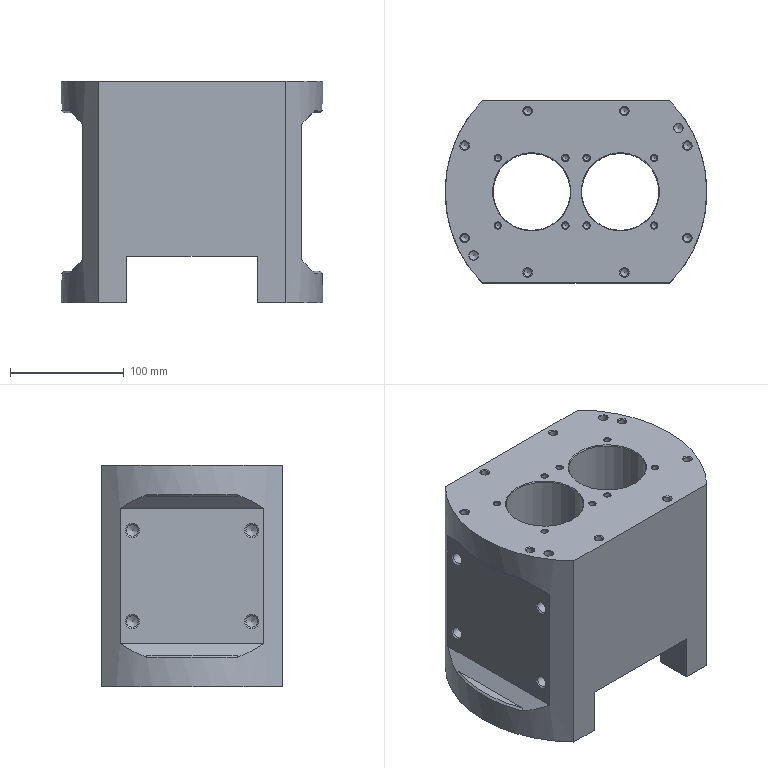NC program | NX | posted with a generic post | part box 230 x 160 x 195 mm
Lines 133 to 1425 of 1674, first 1007 of 1289 lines:
(HOLE_MILLING , TOOL : D35R.5)
N228 T09 M6
N230 G54
N232 G17 G0 G90 X-39. Y0. B0. C0. S1500 M3
N234 G43 Z30. H9
N236 Z1.
N238 G94 G3 X-30.825 Y-8.175 R8.175 F1200.
N240 X-22.65 Y0. R8.175
N242 X-22.65 Y0. Z0.75 I-16.35 J0.
N244 X-22.65 Y0. Z0.5 I-16.35 J0.
N246 X-22.65 Y0. Z0.25 I-16.35 J0.
N248 X-22.65 Y0. Z0. I-16.35 J0.
N250 X-22.65 Y0. Z-0.25 I-16.35 J0.
N252 X-22.65 Y0. Z-0.5 I-16.35 J0.
N254 X-22.65 Y0. Z-0.75 I-16.35 J0.
N256 X-22.65 Y0. Z-1. I-16.35 J0.
N258 X-22.65 Y0. Z-1.25 I-16.35 J0.
N260 X-22.65 Y0. Z-1.5 I-16.35 J0.
N262 X-22.65 Y0. Z-1.75 I-16.35 J0.
N264 X-22.65 Y0. Z-2. I-16.35 J0.
N266 X-22.65 Y0. Z-2.25 I-16.35 J0.
N268 X-22.65 Y0. Z-2.5 I-16.35 J0.
N270 X-22.65 Y0. Z-2.75 I-16.35 J0.
N272 X-22.65 Y0. Z-3. I-16.35 J0.
N274 X-22.65 Y0. Z-3.25 I-16.35 J0.
N276 X-22.65 Y0. Z-3.5 I-16.35 J0.
N278 X-22.65 Y0. Z-3.75 I-16.35 J0.
N280 X-22.65 Y0. Z-4. I-16.35 J0.
N282 X-22.65 Y0. Z-4.25 I-16.35 J0.
N284 X-22.65 Y0. Z-4.5 I-16.35 J0.
N286 X-22.65 Y0. Z-4.75 I-16.35 J0.
N288 X-22.65 Y0. Z-5. I-16.35 J0.
N290 X-22.65 Y0. Z-5.25 I-16.35 J0.
N292 X-22.65 Y0. Z-5.5 I-16.35 J0.
N294 X-22.65 Y0. Z-5.75 I-16.35 J0.
N296 X-22.65 Y0. Z-6. I-16.35 J0.
N298 X-22.65 Y0. Z-6.25 I-16.35 J0.
N300 X-22.65 Y0. Z-6.5 I-16.35 J0.
N302 X-22.65 Y0. Z-6.75 I-16.35 J0.
N304 X-22.65 Y0. Z-7. I-16.35 J0.
N306 X-22.65 Y0. Z-7.25 I-16.35 J0.
N308 X-22.65 Y0. Z-7.5 I-16.35 J0.
N310 X-22.65 Y0. Z-7.75 I-16.35 J0.
N312 X-22.65 Y0. Z-8. I-16.35 J0.
N314 X-22.65 Y0. Z-8.25 I-16.35 J0.
N316 X-22.65 Y0. Z-8.5 I-16.35 J0.
N318 X-22.65 Y0. Z-8.75 I-16.35 J0.
N320 X-22.65 Y0. Z-9. I-16.35 J0.
N322 X-22.65 Y0. Z-9.25 I-16.35 J0.
N324 X-22.65 Y0. Z-9.5 I-16.35 J0.
N326 X-22.65 Y0. Z-9.75 I-16.35 J0.
N328 X-22.65 Y0. Z-10. I-16.35 J0.
N330 X-22.65 Y0. Z-10.25 I-16.35 J0.
N332 X-22.65 Y0. Z-10.5 I-16.35 J0.
N334 X-22.65 Y0. Z-10.75 I-16.35 J0.
N336 X-22.65 Y0. Z-11. I-16.35 J0.
N338 X-22.65 Y0. Z-11.25 I-16.35 J0.
N340 X-22.65 Y0. Z-11.5 I-16.35 J0.
N342 X-22.65 Y0. Z-11.75 I-16.35 J0.
N344 X-22.65 Y0. Z-12. I-16.35 J0.
N346 X-22.65 Y0. Z-12.25 I-16.35 J0.
N348 X-22.65 Y0. Z-12.5 I-16.35 J0.
N350 X-22.65 Y0. Z-12.75 I-16.35 J0.
N352 X-22.65 Y0. Z-13. I-16.35 J0.
N354 X-22.65 Y0. Z-13.25 I-16.35 J0.
N356 X-22.65 Y0. Z-13.5 I-16.35 J0.
N358 X-22.65 Y0. Z-13.75 I-16.35 J0.
N360 X-22.65 Y0. Z-14. I-16.35 J0.
N362 X-22.65 Y0. Z-14.25 I-16.35 J0.
N364 X-22.65 Y0. Z-14.5 I-16.35 J0.
N366 X-22.65 Y0. Z-14.75 I-16.35 J0.
N368 X-22.65 Y0. Z-15. I-16.35 J0.
N370 X-22.65 Y0. Z-15.25 I-16.35 J0.
N372 X-22.65 Y0. Z-15.5 I-16.35 J0.
N374 X-22.65 Y0. Z-15.75 I-16.35 J0.
N376 X-22.65 Y0. Z-16. I-16.35 J0.
N378 X-22.65 Y0. Z-16.25 I-16.35 J0.
N380 X-22.65 Y0. Z-16.5 I-16.35 J0.
N382 X-22.65 Y0. Z-16.75 I-16.35 J0.
N384 X-22.65 Y0. Z-17. I-16.35 J0.
N386 X-22.65 Y0. Z-17.25 I-16.35 J0.
N388 X-22.65 Y0. Z-17.5 I-16.35 J0.
N390 X-22.65 Y0. Z-17.75 I-16.35 J0.
N392 X-22.65 Y0. Z-18. I-16.35 J0.
N394 X-22.65 Y0. Z-18.25 I-16.35 J0.
N396 X-22.65 Y0. Z-18.5 I-16.35 J0.
N398 X-22.65 Y0. Z-18.75 I-16.35 J0.
N400 X-22.65 Y0. Z-19. I-16.35 J0.
N402 X-22.65 Y0. Z-19.25 I-16.35 J0.
N404 X-22.65 Y0. Z-19.5 I-16.35 J0.
N406 X-22.65 Y0. Z-19.75 I-16.35 J0.
N408 X-22.65 Y0. Z-20. I-16.35 J0.
N410 X-22.65 Y0. Z-20.25 I-16.35 J0.
N412 X-22.65 Y0. Z-20.5 I-16.35 J0.
N414 X-22.65 Y0. Z-20.75 I-16.35 J0.
N416 X-22.65 Y0. Z-21. I-16.35 J0.
N418 X-22.65 Y0. Z-21.25 I-16.35 J0.
N420 X-22.65 Y0. Z-21.5 I-16.35 J0.
N422 X-22.65 Y0. Z-21.75 I-16.35 J0.
N424 X-22.65 Y0. Z-22. I-16.35 J0.
N426 X-22.65 Y0. Z-22.25 I-16.35 J0.
N428 X-22.65 Y0. Z-22.5 I-16.35 J0.
N430 X-22.65 Y0. Z-22.75 I-16.35 J0.
N432 X-22.65 Y0. Z-23. I-16.35 J0.
N434 X-22.65 Y0. Z-23.25 I-16.35 J0.
N436 X-22.65 Y0. Z-23.5 I-16.35 J0.
N438 X-22.65 Y0. Z-23.75 I-16.35 J0.
N440 X-22.65 Y0. Z-24. I-16.35 J0.
N442 X-22.65 Y0. Z-24.25 I-16.35 J0.
N444 X-22.65 Y0. Z-24.5 I-16.35 J0.
N446 X-22.65 Y0. Z-24.75 I-16.35 J0.
N448 X-22.65 Y0. Z-25. I-16.35 J0.
N450 X-22.65 Y0. Z-25.25 I-16.35 J0.
N452 X-22.65 Y0. Z-25.5 I-16.35 J0.
N454 X-22.65 Y0. Z-25.75 I-16.35 J0.
N456 X-22.65 Y0. Z-26. I-16.35 J0.
N458 X-22.65 Y0. Z-26.25 I-16.35 J0.
N460 X-22.65 Y0. Z-26.5 I-16.35 J0.
N462 X-22.65 Y0. Z-26.75 I-16.35 J0.
N464 X-22.65 Y0. Z-27. I-16.35 J0.
N466 X-22.65 Y0. Z-27.25 I-16.35 J0.
N468 X-22.65 Y0. Z-27.5 I-16.35 J0.
N470 X-22.65 Y0. Z-27.75 I-16.35 J0.
N472 X-22.65 Y0. Z-28. I-16.35 J0.
N474 X-22.65 Y0. Z-28.25 I-16.35 J0.
N476 X-22.65 Y0. Z-28.5 I-16.35 J0.
N478 X-22.65 Y0. Z-28.75 I-16.35 J0.
N480 X-22.65 Y0. Z-29. I-16.35 J0.
N482 X-22.65 Y0. Z-29.25 I-16.35 J0.
N484 X-22.65 Y0. Z-29.5 I-16.35 J0.
N486 X-22.65 Y0. Z-29.75 I-16.35 J0.
N488 X-22.65 Y0. Z-30. I-16.35 J0.
N490 X-22.65 Y0. Z-30.25 I-16.35 J0.
N492 X-22.65 Y0. Z-30.5 I-16.35 J0.
N494 X-22.65 Y0. Z-30.75 I-16.35 J0.
N496 X-22.65 Y0. Z-31. I-16.35 J0.
N498 X-22.65 Y0. Z-31.25 I-16.35 J0.
N500 X-22.65 Y0. Z-31.5 I-16.35 J0.
N502 X-22.65 Y0. Z-31.75 I-16.35 J0.
N504 X-22.65 Y0. Z-32. I-16.35 J0.
N506 X-22.65 Y0. Z-32.25 I-16.35 J0.
N508 X-22.65 Y0. Z-32.5 I-16.35 J0.
N510 X-22.65 Y0. Z-32.75 I-16.35 J0.
N512 X-22.65 Y0. Z-33. I-16.35 J0.
N514 X-22.65 Y0. Z-33.25 I-16.35 J0.
N516 X-22.65 Y0. Z-33.5 I-16.35 J0.
N518 X-22.65 Y0. Z-33.75 I-16.35 J0.
N520 X-22.65 Y0. Z-34. I-16.35 J0.
N522 X-22.65 Y0. Z-34.25 I-16.35 J0.
N524 X-22.65 Y0. Z-34.5 I-16.35 J0.
N526 X-22.65 Y0. Z-34.75 I-16.35 J0.
N528 X-22.65 Y0. Z-35. I-16.35 J0.
N530 X-22.65 Y0. Z-35.25 I-16.35 J0.
N532 X-22.65 Y0. Z-35.5 I-16.35 J0.
N534 X-22.65 Y0. Z-35.75 I-16.35 J0.
N536 X-22.65 Y0. Z-36. I-16.35 J0.
N538 X-22.65 Y0. Z-36.25 I-16.35 J0.
N540 X-22.65 Y0. Z-36.5 I-16.35 J0.
N542 X-22.65 Y0. Z-36.75 I-16.35 J0.
N544 X-22.65 Y0. Z-37. I-16.35 J0.
N546 X-22.65 Y0. Z-37.25 I-16.35 J0.
N548 X-22.65 Y0. Z-37.5 I-16.35 J0.
N550 X-22.65 Y0. Z-37.75 I-16.35 J0.
N552 X-22.65 Y0. Z-38. I-16.35 J0.
N554 X-22.65 Y0. Z-38.25 I-16.35 J0.
N556 X-22.65 Y0. Z-38.5 I-16.35 J0.
N558 X-22.65 Y0. Z-38.75 I-16.35 J0.
N560 X-22.65 Y0. Z-39. I-16.35 J0.
N562 X-22.65 Y0. Z-39.25 I-16.35 J0.
N564 X-22.65 Y0. Z-39.5 I-16.35 J0.
N566 X-22.65 Y0. Z-39.75 I-16.35 J0.
N568 X-22.65 Y0. Z-40. I-16.35 J0.
N570 X-22.65 Y0. Z-40.25 I-16.35 J0.
N572 X-22.65 Y0. Z-40.5 I-16.35 J0.
N574 X-22.65 Y0. Z-40.75 I-16.35 J0.
N576 X-22.65 Y0. Z-41. I-16.35 J0.
N578 X-22.65 Y0. Z-41.25 I-16.35 J0.
N580 X-22.65 Y0. Z-41.5 I-16.35 J0.
N582 X-22.65 Y0. Z-41.75 I-16.35 J0.
N584 X-22.65 Y0. Z-42. I-16.35 J0.
N586 X-22.65 Y0. Z-42.25 I-16.35 J0.
N588 X-22.65 Y0. Z-42.5 I-16.35 J0.
N590 X-22.65 Y0. Z-42.75 I-16.35 J0.
N592 X-22.65 Y0. Z-43. I-16.35 J0.
N594 X-22.65 Y0. Z-43.25 I-16.35 J0.
N596 X-22.65 Y0. Z-43.5 I-16.35 J0.
N598 X-22.65 Y0. Z-43.75 I-16.35 J0.
N600 X-22.65 Y0. Z-44. I-16.35 J0.
N602 X-22.65 Y0. Z-44.25 I-16.35 J0.
N604 X-22.65 Y0. Z-44.5 I-16.35 J0.
N606 X-22.65 Y0. Z-44.75 I-16.35 J0.
N608 X-22.65 Y0. Z-45. I-16.35 J0.
N610 X-22.65 Y0. Z-45.25 I-16.35 J0.
N612 X-22.65 Y0. Z-45.5 I-16.35 J0.
N614 X-22.65 Y0. Z-45.75 I-16.35 J0.
N616 X-22.65 Y0. Z-46. I-16.35 J0.
N618 X-22.65 Y0. Z-46.25 I-16.35 J0.
N620 X-22.65 Y0. Z-46.5 I-16.35 J0.
N622 X-22.65 Y0. Z-46.75 I-16.35 J0.
N624 X-22.65 Y0. Z-47. I-16.35 J0.
N626 X-22.65 Y0. Z-47.25 I-16.35 J0.
N628 X-22.65 Y0. Z-47.5 I-16.35 J0.
N630 X-22.65 Y0. Z-47.75 I-16.35 J0.
N632 X-22.65 Y0. Z-48. I-16.35 J0.
N634 X-22.65 Y0. Z-48.25 I-16.35 J0.
N636 X-22.65 Y0. Z-48.5 I-16.35 J0.
N638 X-22.65 Y0. Z-48.75 I-16.35 J0.
N640 X-22.65 Y0. Z-49. I-16.35 J0.
N642 X-22.65 Y0. Z-49.25 I-16.35 J0.
N644 X-22.65 Y0. Z-49.5 I-16.35 J0.
N646 X-22.65 Y0. Z-49.75 I-16.35 J0.
N648 X-22.65 Y0. Z-50. I-16.35 J0.
N650 X-22.65 Y0. Z-50.25 I-16.35 J0.
N652 X-22.65 Y0. Z-50.5 I-16.35 J0.
N654 X-22.65 Y0. Z-50.75 I-16.35 J0.
N656 X-22.65 Y0. Z-51. I-16.35 J0.
N658 X-22.65 Y0. Z-51.25 I-16.35 J0.
N660 X-22.65 Y0. Z-51.5 I-16.35 J0.
N662 X-22.65 Y0. Z-51.75 I-16.35 J0.
N664 X-22.65 Y0. Z-52. I-16.35 J0.
N666 X-22.65 Y0. Z-52.25 I-16.35 J0.
N668 X-22.65 Y0. Z-52.5 I-16.35 J0.
N670 X-22.65 Y0. Z-52.75 I-16.35 J0.
N672 X-22.65 Y0. Z-53. I-16.35 J0.
N674 X-22.65 Y0. Z-53.25 I-16.35 J0.
N676 X-22.65 Y0. Z-53.5 I-16.35 J0.
N678 X-22.65 Y0. Z-53.75 I-16.35 J0.
N680 X-22.65 Y0. Z-54. I-16.35 J0.
N682 X-22.65 Y0. Z-54.25 I-16.35 J0.
N684 X-22.65 Y0. Z-54.5 I-16.35 J0.
N686 X-22.65 Y0. Z-54.75 I-16.35 J0.
N688 X-22.65 Y0. Z-55. I-16.35 J0.
N690 X-22.65 Y0. Z-55.25 I-16.35 J0.
N692 X-22.65 Y0. Z-55.5 I-16.35 J0.
N694 X-22.65 Y0. Z-55.75 I-16.35 J0.
N696 X-22.65 Y0. Z-56. I-16.35 J0.
N698 X-22.65 Y0. Z-56.25 I-16.35 J0.
N700 X-22.65 Y0. Z-56.5 I-16.35 J0.
N702 X-22.65 Y0. Z-56.75 I-16.35 J0.
N704 X-22.65 Y0. Z-57. I-16.35 J0.
N706 X-22.65 Y0. Z-57.25 I-16.35 J0.
N708 X-22.65 Y0. Z-57.5 I-16.35 J0.
N710 X-22.65 Y0. Z-57.75 I-16.35 J0.
N712 X-22.65 Y0. Z-58. I-16.35 J0.
N714 X-22.65 Y0. Z-58.25 I-16.35 J0.
N716 X-22.65 Y0. Z-58.5 I-16.35 J0.
N718 X-22.65 Y0. Z-58.75 I-16.35 J0.
N720 X-22.65 Y0. Z-59. I-16.35 J0.
N722 X-22.65 Y0. Z-59.25 I-16.35 J0.
N724 X-22.65 Y0. Z-59.5 I-16.35 J0.
N726 X-22.65 Y0. Z-59.75 I-16.35 J0.
N728 X-22.65 Y0. Z-60. I-16.35 J0.
N730 X-22.65 Y0. Z-60.25 I-16.35 J0.
N732 X-22.65 Y0. Z-60.5 I-16.35 J0.
N734 X-22.65 Y0. Z-60.75 I-16.35 J0.
N736 X-22.65 Y0. Z-61. I-16.35 J0.
N738 X-22.65 Y0. Z-61.25 I-16.35 J0.
N740 X-22.65 Y0. Z-61.5 I-16.35 J0.
N742 X-22.65 Y0. Z-61.75 I-16.35 J0.
N744 X-22.65 Y0. Z-62. I-16.35 J0.
N746 X-22.65 Y0. Z-62.25 I-16.35 J0.
N748 X-22.65 Y0. Z-62.5 I-16.35 J0.
N750 X-22.65 Y0. Z-62.75 I-16.35 J0.
N752 X-22.65 Y0. Z-63. I-16.35 J0.
N754 X-22.65 Y0. Z-63.25 I-16.35 J0.
N756 X-22.65 Y0. Z-63.5 I-16.35 J0.
N758 X-22.65 Y0. Z-63.75 I-16.35 J0.
N760 X-22.65 Y0. Z-64. I-16.35 J0.
N762 X-22.65 Y0. Z-64.25 I-16.35 J0.
N764 X-22.65 Y0. Z-64.5 I-16.35 J0.
N766 X-22.65 Y0. Z-64.75 I-16.35 J0.
N768 X-22.65 Y0. Z-65. I-16.35 J0.
N770 X-22.65 Y0. Z-65.25 I-16.35 J0.
N772 X-22.65 Y0. Z-65.5 I-16.35 J0.
N774 X-22.65 Y0. Z-65.75 I-16.35 J0.
N776 X-22.65 Y0. Z-66. I-16.35 J0.
N778 X-22.65 Y0. Z-66.25 I-16.35 J0.
N780 X-22.65 Y0. Z-66.5 I-16.35 J0.
N782 X-22.65 Y0. Z-66.75 I-16.35 J0.
N784 X-22.65 Y0. Z-67. I-16.35 J0.
N786 X-22.65 Y0. Z-67.25 I-16.35 J0.
N788 X-22.65 Y0. Z-67.5 I-16.35 J0.
N790 X-22.65 Y0. Z-67.75 I-16.35 J0.
N792 X-22.65 Y0. Z-68. I-16.35 J0.
N794 X-22.65 Y0. Z-68.25 I-16.35 J0.
N796 X-22.65 Y0. Z-68.5 I-16.35 J0.
N798 X-22.65 Y0. Z-68.75 I-16.35 J0.
N800 X-22.65 Y0. Z-69. I-16.35 J0.
N802 X-22.65 Y0. Z-69.25 I-16.35 J0.
N804 X-22.65 Y0. Z-69.5 I-16.35 J0.
N806 X-22.65 Y0. Z-69.75 I-16.35 J0.
N808 X-22.65 Y0. Z-70. I-16.35 J0.
N810 X-22.65 Y0. Z-70.25 I-16.35 J0.
N812 X-22.65 Y0. Z-70.5 I-16.35 J0.
N814 X-22.65 Y0. Z-70.75 I-16.35 J0.
N816 X-22.65 Y0. Z-71. I-16.35 J0.
N818 X-22.65 Y0. Z-71.25 I-16.35 J0.
N820 X-22.65 Y0. Z-71.5 I-16.35 J0.
N822 X-22.65 Y0. Z-71.75 I-16.35 J0.
N824 X-22.65 Y0. Z-72. I-16.35 J0.
N826 X-22.65 Y0. Z-72.25 I-16.35 J0.
N828 X-22.65 Y0. Z-72.5 I-16.35 J0.
N830 X-22.65 Y0. Z-72.75 I-16.35 J0.
N832 X-22.65 Y0. Z-73. I-16.35 J0.
N834 X-22.65 Y0. Z-73.25 I-16.35 J0.
N836 X-22.65 Y0. Z-73.5 I-16.35 J0.
N838 X-22.65 Y0. Z-73.75 I-16.35 J0.
N840 X-22.65 Y0. Z-74. I-16.35 J0.
N842 X-22.65 Y0. Z-74.25 I-16.35 J0.
N844 X-22.65 Y0. Z-74.5 I-16.35 J0.
N846 X-22.65 Y0. Z-74.75 I-16.35 J0.
N848 X-22.65 Y0. Z-75. I-16.35 J0.
N850 X-22.65 Y0. Z-75.25 I-16.35 J0.
N852 X-22.65 Y0. Z-75.5 I-16.35 J0.
N854 X-22.65 Y0. Z-75.75 I-16.35 J0.
N856 X-22.65 Y0. Z-76. I-16.35 J0.
N858 X-22.65 Y0. Z-76.25 I-16.35 J0.
N860 X-22.65 Y0. Z-76.5 I-16.35 J0.
N862 X-22.65 Y0. Z-76.75 I-16.35 J0.
N864 X-22.65 Y0. Z-77. I-16.35 J0.
N866 X-22.65 Y0. Z-77.25 I-16.35 J0.
N868 X-22.65 Y0. Z-77.5 I-16.35 J0.
N870 X-22.65 Y0. Z-77.75 I-16.35 J0.
N872 X-22.65 Y0. Z-78. I-16.35 J0.
N874 X-22.65 Y0. Z-78.25 I-16.35 J0.
N876 X-22.65 Y0. Z-78.5 I-16.35 J0.
N878 X-22.65 Y0. Z-78.75 I-16.35 J0.
N880 X-22.65 Y0. Z-79. I-16.35 J0.
N882 X-22.65 Y0. Z-79.25 I-16.35 J0.
N884 X-22.65 Y0. Z-79.5 I-16.35 J0.
N886 X-22.65 Y0. Z-79.75 I-16.35 J0.
N888 X-22.65 Y0. Z-80. I-16.35 J0.
N890 X-22.65 Y0. Z-80.25 I-16.35 J0.
N892 X-22.65 Y0. Z-80.5 I-16.35 J0.
N894 X-22.65 Y0. Z-80.75 I-16.35 J0.
N896 X-22.65 Y0. Z-81. I-16.35 J0.
N898 X-22.65 Y0. Z-81.25 I-16.35 J0.
N900 X-22.65 Y0. Z-81.5 I-16.35 J0.
N902 X-22.65 Y0. Z-81.75 I-16.35 J0.
N904 X-22.65 Y0. Z-82. I-16.35 J0.
N906 X-22.65 Y0. Z-82.25 I-16.35 J0.
N908 X-22.65 Y0. Z-82.5 I-16.35 J0.
N910 X-22.65 Y0. Z-82.75 I-16.35 J0.
N912 X-22.65 Y0. Z-83. I-16.35 J0.
N914 X-22.65 Y0. Z-83.25 I-16.35 J0.
N916 X-22.65 Y0. Z-83.5 I-16.35 J0.
N918 X-22.65 Y0. Z-83.75 I-16.35 J0.
N920 X-22.65 Y0. Z-84. I-16.35 J0.
N922 X-22.65 Y0. Z-84.25 I-16.35 J0.
N924 X-22.65 Y0. Z-84.5 I-16.35 J0.
N926 X-22.65 Y0. Z-84.75 I-16.35 J0.
N928 X-22.65 Y0. Z-85. I-16.35 J0.
N930 X-22.65 Y0. Z-85.25 I-16.35 J0.
N932 X-22.65 Y0. Z-85.5 I-16.35 J0.
N934 X-22.65 Y0. Z-85.75 I-16.35 J0.
N936 X-22.65 Y0. Z-86. I-16.35 J0.
N938 X-22.65 Y0. Z-86.25 I-16.35 J0.
N940 X-22.65 Y0. Z-86.5 I-16.35 J0.
N942 X-22.65 Y0. Z-86.75 I-16.35 J0.
N944 X-22.65 Y0. Z-87. I-16.35 J0.
N946 X-22.65 Y0. Z-87.25 I-16.35 J0.
N948 X-22.65 Y0. Z-87.5 I-16.35 J0.
N950 X-22.65 Y0. Z-87.75 I-16.35 J0.
N952 X-22.65 Y0. Z-88. I-16.35 J0.
N954 X-22.65 Y0. Z-88.25 I-16.35 J0.
N956 X-22.65 Y0. Z-88.5 I-16.35 J0.
N958 X-22.65 Y0. Z-88.75 I-16.35 J0.
N960 X-22.65 Y0. Z-89. I-16.35 J0.
N962 X-22.65 Y0. Z-89.25 I-16.35 J0.
N964 X-22.65 Y0. Z-89.5 I-16.35 J0.
N966 X-22.65 Y0. Z-89.75 I-16.35 J0.
N968 X-22.65 Y0. Z-90. I-16.35 J0.
N970 X-22.65 Y0. Z-90.25 I-16.35 J0.
N972 X-22.65 Y0. Z-90.5 I-16.35 J0.
N974 X-22.65 Y0. Z-90.75 I-16.35 J0.
N976 X-22.65 Y0. Z-91. I-16.35 J0.
N978 X-22.65 Y0. Z-91.25 I-16.35 J0.
N980 X-22.65 Y0. Z-91.5 I-16.35 J0.
N982 X-22.65 Y0. Z-91.75 I-16.35 J0.
N984 X-22.65 Y0. Z-92. I-16.35 J0.
N986 X-22.65 Y0. Z-92.25 I-16.35 J0.
N988 X-22.65 Y0. Z-92.5 I-16.35 J0.
N990 X-22.65 Y0. Z-92.75 I-16.35 J0.
N992 X-22.65 Y0. Z-93. I-16.35 J0.
N994 X-22.65 Y0. Z-93.25 I-16.35 J0.
N996 X-22.65 Y0. Z-93.5 I-16.35 J0.
N998 X-22.65 Y0. Z-93.75 I-16.35 J0.
N1000 X-22.65 Y0. Z-94. I-16.35 J0.
N1002 X-22.65 Y0. Z-94.25 I-16.35 J0.
N1004 X-22.65 Y0. Z-94.5 I-16.35 J0.
N1006 X-22.65 Y0. Z-94.75 I-16.35 J0.
N1008 X-22.65 Y0. Z-95. I-16.35 J0.
N1010 X-22.65 Y0. Z-95.25 I-16.35 J0.
N1012 X-22.65 Y0. Z-95.5 I-16.35 J0.
N1014 X-22.65 Y0. Z-95.75 I-16.35 J0.
N1016 X-22.65 Y0. Z-96. I-16.35 J0.
N1018 X-22.65 Y0. Z-96.25 I-16.35 J0.
N1020 X-22.65 Y0. Z-96.5 I-16.35 J0.
N1022 X-22.65 Y0. Z-96.75 I-16.35 J0.
N1024 X-22.65 Y0. Z-97. I-16.35 J0.
N1026 X-22.65 Y0. Z-97.25 I-16.35 J0.
N1028 X-22.65 Y0. Z-97.5 I-16.35 J0.
N1030 X-22.65 Y0. Z-97.75 I-16.35 J0.
N1032 X-22.65 Y0. Z-98. I-16.35 J0.
N1034 X-22.65 Y0. Z-98.25 I-16.35 J0.
N1036 X-22.65 Y0. Z-98.5 I-16.35 J0.
N1038 X-22.65 Y0. Z-98.75 I-16.35 J0.
N1040 X-22.65 Y0. Z-99. I-16.35 J0.
N1042 X-22.65 Y0. Z-99.25 I-16.35 J0.
N1044 X-22.65 Y0. Z-99.5 I-16.35 J0.
N1046 X-22.65 Y0. Z-99.75 I-16.35 J0.
N1048 X-22.65 Y0. Z-100. I-16.35 J0.
N1050 X-22.65 Y0. Z-100.25 I-16.35 J0.
N1052 X-22.65 Y0. Z-100.5 I-16.35 J0.
N1054 X-22.65 Y0. Z-100.75 I-16.35 J0.
N1056 X-22.65 Y0. Z-101. I-16.35 J0.
N1058 X-22.65 Y0. Z-101.25 I-16.35 J0.
N1060 X-22.65 Y0. Z-101.5 I-16.35 J0.
N1062 X-22.65 Y0. Z-101.75 I-16.35 J0.
N1064 X-22.65 Y0. Z-102. I-16.35 J0.
N1066 X-22.65 Y0. Z-102.25 I-16.35 J0.
N1068 X-22.65 Y0. Z-102.5 I-16.35 J0.
N1070 X-22.65 Y0. Z-102.75 I-16.35 J0.
N1072 X-22.65 Y0. Z-103. I-16.35 J0.
N1074 X-22.65 Y0. Z-103.25 I-16.35 J0.
N1076 X-22.65 Y0. Z-103.5 I-16.35 J0.
N1078 X-22.65 Y0. Z-103.75 I-16.35 J0.
N1080 X-22.65 Y0. Z-104. I-16.35 J0.
N1082 X-22.65 Y0. Z-104.25 I-16.35 J0.
N1084 X-22.65 Y0. Z-104.5 I-16.35 J0.
N1086 X-22.65 Y0. Z-104.75 I-16.35 J0.
N1088 X-22.65 Y0. Z-105. I-16.35 J0.
N1090 X-22.65 Y0. Z-105.25 I-16.35 J0.
N1092 X-22.65 Y0. Z-105.5 I-16.35 J0.
N1094 X-22.65 Y0. Z-105.75 I-16.35 J0.
N1096 X-22.65 Y0. Z-106. I-16.35 J0.
N1098 X-22.65 Y0. Z-106.25 I-16.35 J0.
N1100 X-22.65 Y0. Z-106.5 I-16.35 J0.
N1102 X-22.65 Y0. Z-106.75 I-16.35 J0.
N1104 X-22.65 Y0. Z-107. I-16.35 J0.
N1106 X-22.65 Y0. Z-107.25 I-16.35 J0.
N1108 X-22.65 Y0. Z-107.5 I-16.35 J0.
N1110 X-22.65 Y0. Z-107.75 I-16.35 J0.
N1112 X-22.65 Y0. Z-108. I-16.35 J0.
N1114 X-22.65 Y0. Z-108.25 I-16.35 J0.
N1116 X-22.65 Y0. Z-108.5 I-16.35 J0.
N1118 X-22.65 Y0. Z-108.75 I-16.35 J0.
N1120 X-22.65 Y0. Z-109. I-16.35 J0.
N1122 X-22.65 Y0. Z-109.25 I-16.35 J0.
N1124 X-22.65 Y0. Z-109.5 I-16.35 J0.
N1126 X-22.65 Y0. Z-109.75 I-16.35 J0.
N1128 X-22.65 Y0. Z-110. I-16.35 J0.
N1130 X-22.65 Y0. Z-110.25 I-16.35 J0.
N1132 X-22.65 Y0. Z-110.5 I-16.35 J0.
N1134 X-22.65 Y0. Z-110.75 I-16.35 J0.
N1136 X-22.65 Y0. Z-111. I-16.35 J0.
N1138 X-22.65 Y0. Z-111.25 I-16.35 J0.
N1140 X-22.65 Y0. Z-111.5 I-16.35 J0.
N1142 X-22.65 Y0. Z-111.75 I-16.35 J0.
N1144 X-22.65 Y0. Z-112. I-16.35 J0.
N1146 X-22.65 Y0. Z-112.25 I-16.35 J0.
N1148 X-22.65 Y0. Z-112.5 I-16.35 J0.
N1150 X-22.65 Y0. Z-112.75 I-16.35 J0.
N1152 X-22.65 Y0. Z-113. I-16.35 J0.
N1154 X-22.65 Y0. Z-113.25 I-16.35 J0.
N1156 X-22.65 Y0. Z-113.5 I-16.35 J0.
N1158 X-22.65 Y0. Z-113.75 I-16.35 J0.
N1160 X-22.65 Y0. Z-114. I-16.35 J0.
N1162 X-22.65 Y0. Z-114.25 I-16.35 J0.
N1164 X-22.65 Y0. Z-114.5 I-16.35 J0.
N1166 X-22.65 Y0. Z-114.75 I-16.35 J0.
N1168 X-22.65 Y0. Z-115. I-16.35 J0.
N1170 X-22.65 Y0. Z-115.25 I-16.35 J0.
N1172 X-22.65 Y0. Z-115.5 I-16.35 J0.
N1174 X-22.65 Y0. Z-115.75 I-16.35 J0.
N1176 X-22.65 Y0. Z-116. I-16.35 J0.
N1178 X-22.65 Y0. Z-116.25 I-16.35 J0.
N1180 X-22.65 Y0. Z-116.5 I-16.35 J0.
N1182 X-22.65 Y0. Z-116.75 I-16.35 J0.
N1184 X-22.65 Y0. Z-117. I-16.35 J0.
N1186 X-22.65 Y0. Z-117.25 I-16.35 J0.
N1188 X-22.65 Y0. Z-117.5 I-16.35 J0.
N1190 X-22.65 Y0. Z-117.75 I-16.35 J0.
N1192 X-22.65 Y0. Z-118. I-16.35 J0.
N1194 X-22.65 Y0. Z-118.25 I-16.35 J0.
N1196 X-22.65 Y0. Z-118.5 I-16.35 J0.
N1198 X-22.65 Y0. Z-118.75 I-16.35 J0.
N1200 X-22.65 Y0. Z-119. I-16.35 J0.
N1202 X-22.65 Y0. Z-119.25 I-16.35 J0.
N1204 X-22.65 Y0. Z-119.5 I-16.35 J0.
N1206 X-22.65 Y0. Z-119.75 I-16.35 J0.
N1208 X-22.65 Y0. Z-120. I-16.35 J0.
N1210 X-22.65 Y0. Z-120.25 I-16.35 J0.
N1212 X-22.65 Y0. Z-120.5 I-16.35 J0.
N1214 X-22.65 Y0. Z-120.75 I-16.35 J0.
N1216 X-22.65 Y0. Z-121. I-16.35 J0.
N1218 X-22.65 Y0. Z-121.25 I-16.35 J0.
N1220 X-22.65 Y0. Z-121.5 I-16.35 J0.
N1222 X-22.65 Y0. Z-121.75 I-16.35 J0.
N1224 X-22.65 Y0. Z-122. I-16.35 J0.
N1226 X-22.65 Y0. Z-122.25 I-16.35 J0.
N1228 X-22.65 Y0. Z-122.5 I-16.35 J0.
N1230 X-22.65 Y0. Z-122.75 I-16.35 J0.
N1232 X-22.65 Y0. Z-123. I-16.35 J0.
N1234 X-22.65 Y0. Z-123.25 I-16.35 J0.
N1236 X-22.65 Y0. Z-123.5 I-16.35 J0.
N1238 X-22.65 Y0. Z-123.75 I-16.35 J0.
N1240 X-22.65 Y0. Z-124. I-16.35 J0.
N1242 X-22.65 Y0. Z-124.25 I-16.35 J0.
N1244 X-22.65 Y0. Z-124.5 I-16.35 J0.
N1246 X-22.65 Y0. Z-124.75 I-16.35 J0.
N1248 X-22.65 Y0. Z-125. I-16.35 J0.
N1250 X-22.65 Y0. Z-125.25 I-16.35 J0.
N1252 X-22.65 Y0. Z-125.5 I-16.35 J0.
N1254 X-22.65 Y0. Z-125.75 I-16.35 J0.
N1256 X-22.65 Y0. Z-126. I-16.35 J0.
N1258 X-22.65 Y0. Z-126.25 I-16.35 J0.
N1260 X-22.65 Y0. Z-126.5 I-16.35 J0.
N1262 X-22.65 Y0. Z-126.75 I-16.35 J0.
N1264 X-22.65 Y0. Z-127. I-16.35 J0.
N1266 X-22.65 Y0. Z-127.25 I-16.35 J0.
N1268 X-22.65 Y0. Z-127.5 I-16.35 J0.
N1270 X-22.65 Y0. Z-127.75 I-16.35 J0.
N1272 X-22.65 Y0. Z-128. I-16.35 J0.
N1274 X-22.65 Y0. Z-128.25 I-16.35 J0.
N1276 X-22.65 Y0. Z-128.5 I-16.35 J0.
N1278 X-22.65 Y0. Z-128.75 I-16.35 J0.
N1280 X-22.65 Y0. Z-129. I-16.35 J0.
N1282 X-22.65 Y0. Z-129.25 I-16.35 J0.
N1284 X-22.65 Y0. Z-129.5 I-16.35 J0.
N1286 X-22.65 Y0. Z-129.75 I-16.35 J0.
N1288 X-22.65 Y0. Z-130. I-16.35 J0.
N1290 X-22.65 Y0. Z-130.25 I-16.35 J0.
N1292 X-22.65 Y0. Z-130.5 I-16.35 J0.
N1294 X-22.65 Y0. Z-130.75 I-16.35 J0.
N1296 X-22.65 Y0. Z-131. I-16.35 J0.
N1298 X-22.65 Y0. Z-131.25 I-16.35 J0.
N1300 X-22.65 Y0. Z-131.5 I-16.35 J0.
N1302 X-22.65 Y0. Z-131.75 I-16.35 J0.
N1304 X-22.65 Y0. Z-132. I-16.35 J0.
N1306 X-22.65 Y0. Z-132.25 I-16.35 J0.
N1308 X-22.65 Y0. Z-132.5 I-16.35 J0.
N1310 X-22.65 Y0. Z-132.75 I-16.35 J0.
N1312 X-22.65 Y0. Z-133. I-16.35 J0.
N1314 X-22.65 Y0. Z-133.25 I-16.35 J0.
N1316 X-22.65 Y0. Z-133.5 I-16.35 J0.
N1318 X-22.65 Y0. Z-133.75 I-16.35 J0.
N1320 X-22.65 Y0. Z-134. I-16.35 J0.
N1322 X-22.65 Y0. Z-134.25 I-16.35 J0.
N1324 X-22.65 Y0. Z-134.5 I-16.35 J0.
N1326 X-22.65 Y0. Z-134.75 I-16.35 J0.
N1328 X-22.65 Y0. Z-135. I-16.35 J0.
N1330 X-22.65 Y0. Z-135.25 I-16.35 J0.
N1332 X-22.65 Y0. Z-135.5 I-16.35 J0.
N1334 X-22.65 Y0. Z-135.75 I-16.35 J0.
N1336 X-22.65 Y0. Z-136. I-16.35 J0.
N1338 X-22.65 Y0. Z-136.25 I-16.35 J0.
N1340 X-22.65 Y0. Z-136.5 I-16.35 J0.
N1342 X-22.65 Y0. Z-136.75 I-16.35 J0.
N1344 X-22.65 Y0. Z-137. I-16.35 J0.
N1346 X-22.65 Y0. Z-137.25 I-16.35 J0.
N1348 X-22.65 Y0. Z-137.5 I-16.35 J0.
N1350 X-22.65 Y0. Z-137.75 I-16.35 J0.
N1352 X-22.65 Y0. Z-138. I-16.35 J0.
N1354 X-22.65 Y0. Z-138.25 I-16.35 J0.
N1356 X-22.65 Y0. Z-138.5 I-16.35 J0.
N1358 X-22.65 Y0. Z-138.75 I-16.35 J0.
N1360 X-22.65 Y0. Z-139. I-16.35 J0.
N1362 X-22.65 Y0. Z-139.25 I-16.35 J0.
N1364 X-22.65 Y0. Z-139.5 I-16.35 J0.
N1366 X-22.65 Y0. Z-139.75 I-16.35 J0.
N1368 X-22.65 Y0. Z-140. I-16.35 J0.
N1370 X-22.65 Y0. Z-140.25 I-16.35 J0.
N1372 X-22.65 Y0. Z-140.5 I-16.35 J0.
N1374 X-22.65 Y0. Z-140.75 I-16.35 J0.
N1376 X-22.65 Y0. Z-141. I-16.35 J0.
N1378 X-22.65 Y0. Z-141.25 I-16.35 J0.
N1380 X-22.65 Y0. Z-141.5 I-16.35 J0.
N1382 X-22.65 Y0. Z-141.75 I-16.35 J0.
N1384 X-22.65 Y0. Z-142. I-16.35 J0.
N1386 X-22.65 Y0. Z-142.25 I-16.35 J0.
N1388 X-22.65 Y0. Z-142.5 I-16.35 J0.
N1390 X-22.65 Y0. Z-142.75 I-16.35 J0.
N1392 X-22.65 Y0. Z-143. I-16.35 J0.
N1394 X-22.65 Y0. Z-143.25 I-16.35 J0.
N1396 X-22.65 Y0. Z-143.5 I-16.35 J0.
N1398 X-22.65 Y0. Z-143.75 I-16.35 J0.
N1400 X-22.65 Y0. Z-144. I-16.35 J0.
N1402 X-22.65 Y0. Z-144.25 I-16.35 J0.
N1404 X-22.65 Y0. Z-144.5 I-16.35 J0.
N1406 X-22.65 Y0. Z-144.75 I-16.35 J0.
N1408 X-22.65 Y0. Z-145. I-16.35 J0.
N1410 X-22.65 Y0. Z-145.25 I-16.35 J0.
N1412 X-22.65 Y0. Z-145.5 I-16.35 J0.
N1414 X-22.65 Y0. Z-145.75 I-16.35 J0.
N1416 X-22.65 Y0. Z-146. I-16.35 J0.
N1418 X-22.65 Y0. Z-146.25 I-16.35 J0.
N1420 X-22.65 Y0. Z-146.5 I-16.35 J0.
N1422 X-22.65 Y0. Z-146.75 I-16.35 J0.
N1424 X-22.65 Y0. Z-147. I-16.35 J0.
N1426 X-22.65 Y0. Z-147.25 I-16.35 J0.
N1428 X-22.65 Y0. Z-147.5 I-16.35 J0.
N1430 X-22.65 Y0. Z-147.75 I-16.35 J0.
N1432 X-22.65 Y0. Z-148. I-16.35 J0.
N1434 X-22.65 Y0. Z-148.25 I-16.35 J0.
N1436 X-22.65 Y0. Z-148.5 I-16.35 J0.
N1438 X-22.65 Y0. Z-148.75 I-16.35 J0.
N1440 X-22.65 Y0. Z-149. I-16.35 J0.
N1442 X-22.65 Y0. Z-149.25 I-16.35 J0.
N1444 X-22.65 Y0. Z-149.5 I-16.35 J0.
N1446 X-22.65 Y0. Z-149.75 I-16.35 J0.
N1448 X-22.65 Y0. Z-150. I-16.35 J0.
N1450 X-22.65 Y0. Z-150.25 I-16.35 J0.
N1452 X-22.65 Y0. Z-150.5 I-16.35 J0.
N1454 X-22.65 Y0. Z-150.75 I-16.35 J0.
N1456 X-22.65 Y0. Z-151. I-16.35 J0.
N1458 X-22.65 Y0. Z-151.25 I-16.35 J0.
N1460 X-22.65 Y0. Z-151.5 I-16.35 J0.
N1462 X-22.65 Y0. Z-151.75 I-16.35 J0.
N1464 X-22.65 Y0. Z-152. I-16.35 J0.
N1466 X-22.65 Y0. Z-152.25 I-16.35 J0.
N1468 X-22.65 Y0. Z-152.5 I-16.35 J0.
N1470 X-22.65 Y0. Z-152.75 I-16.35 J0.
N1472 X-22.65 Y0. Z-153. I-16.35 J0.
N1474 X-22.65 Y0. Z-153.25 I-16.35 J0.
N1476 X-22.65 Y0. Z-153.5 I-16.35 J0.
N1478 X-22.65 Y0. Z-153.75 I-16.35 J0.
N1480 X-22.65 Y0. Z-154. I-16.35 J0.
N1482 X-22.65 Y0. Z-154.25 I-16.35 J0.
N1484 X-22.65 Y0. Z-154.5 I-16.35 J0.
N1486 X-22.65 Y0. Z-154.75 I-16.35 J0.
N1488 X-22.65 Y0. Z-155. I-16.35 J0.
N1490 X-22.65 Y0. Z-155.25 I-16.35 J0.
N1492 X-22.65 Y0. Z-155.5 I-16.35 J0.
N1494 X-22.65 Y0. Z-155.75 I-16.35 J0.
N1496 X-22.65 Y0. Z-156. I-16.35 J0.
N1498 X-39. Y16.35 R16.35
N1500 X-22.65 Y0. R-16.35
N1502 X-30.825 Y8.175 R8.175
N1504 X-39. Y0. R8.175
N1506 G0 Z30.
N1508 X39.
N1510 Z1.
N1512 G3 X47.175 Y-8.175 R8.175
N1514 X55.35 Y0. R8.175
N1516 X55.35 Y0. Z0.75 I-16.35 J0.
N1518 X55.35 Y0. Z0.5 I-16.35 J0.
N1520 X55.35 Y0. Z0.25 I-16.35 J0.
N1522 X55.35 Y0. Z0. I-16.35 J0.
N1524 X55.35 Y0. Z-0.25 I-16.35 J0.
N1526 X55.35 Y0. Z-0.5 I-16.35 J0.
N1528 X55.35 Y0. Z-0.75 I-16.35 J0.
N1530 X55.35 Y0. Z-1. I-16.35 J0.
N1532 X55.35 Y0. Z-1.25 I-16.35 J0.
N1534 X55.35 Y0. Z-1.5 I-16.35 J0.
N1536 X55.35 Y0. Z-1.75 I-16.35 J0.
N1538 X55.35 Y0. Z-2. I-16.35 J0.
N1540 X55.35 Y0. Z-2.25 I-16.35 J0.
N1542 X55.35 Y0. Z-2.5 I-16.35 J0.
N1544 X55.35 Y0. Z-2.75 I-16.35 J0.
N1546 X55.35 Y0. Z-3. I-16.35 J0.
N1548 X55.35 Y0. Z-3.25 I-16.35 J0.
N1550 X55.35 Y0. Z-3.5 I-16.35 J0.
N1552 X55.35 Y0. Z-3.75 I-16.35 J0.
N1554 X55.35 Y0. Z-4. I-16.35 J0.
N1556 X55.35 Y0. Z-4.25 I-16.35 J0.
N1558 X55.35 Y0. Z-4.5 I-16.35 J0.
N1560 X55.35 Y0. Z-4.75 I-16.35 J0.
N1562 X55.35 Y0. Z-5. I-16.35 J0.
N1564 X55.35 Y0. Z-5.25 I-16.35 J0.
N1566 X55.35 Y0. Z-5.5 I-16.35 J0.
N1568 X55.35 Y0. Z-5.75 I-16.35 J0.
N1570 X55.35 Y0. Z-6. I-16.35 J0.
N1572 X55.35 Y0. Z-6.25 I-16.35 J0.
N1574 X55.35 Y0. Z-6.5 I-16.35 J0.
N1576 X55.35 Y0. Z-6.75 I-16.35 J0.
N1578 X55.35 Y0. Z-7. I-16.35 J0.
N1580 X55.35 Y0. Z-7.25 I-16.35 J0.
N1582 X55.35 Y0. Z-7.5 I-16.35 J0.
N1584 X55.35 Y0. Z-7.75 I-16.35 J0.
N1586 X55.35 Y0. Z-8. I-16.35 J0.
N1588 X55.35 Y0. Z-8.25 I-16.35 J0.
N1590 X55.35 Y0. Z-8.5 I-16.35 J0.
N1592 X55.35 Y0. Z-8.75 I-16.35 J0.
N1594 X55.35 Y0. Z-9. I-16.35 J0.
N1596 X55.35 Y0. Z-9.25 I-16.35 J0.
N1598 X55.35 Y0. Z-9.5 I-16.35 J0.
N1600 X55.35 Y0. Z-9.75 I-16.35 J0.
N1602 X55.35 Y0. Z-10. I-16.35 J0.
N1604 X55.35 Y0. Z-10.25 I-16.35 J0.
N1606 X55.35 Y0. Z-10.5 I-16.35 J0.
N1608 X55.35 Y0. Z-10.75 I-16.35 J0.
N1610 X55.35 Y0. Z-11. I-16.35 J0.
N1612 X55.35 Y0. Z-11.25 I-16.35 J0.
N1614 X55.35 Y0. Z-11.5 I-16.35 J0.
N1616 X55.35 Y0. Z-11.75 I-16.35 J0.
N1618 X55.35 Y0. Z-12. I-16.35 J0.
N1620 X55.35 Y0. Z-12.25 I-16.35 J0.
N1622 X55.35 Y0. Z-12.5 I-16.35 J0.
N1624 X55.35 Y0. Z-12.75 I-16.35 J0.
N1626 X55.35 Y0. Z-13. I-16.35 J0.
N1628 X55.35 Y0. Z-13.25 I-16.35 J0.
N1630 X55.35 Y0. Z-13.5 I-16.35 J0.
N1632 X55.35 Y0. Z-13.75 I-16.35 J0.
N1634 X55.35 Y0. Z-14. I-16.35 J0.
N1636 X55.35 Y0. Z-14.25 I-16.35 J0.
N1638 X55.35 Y0. Z-14.5 I-16.35 J0.
N1640 X55.35 Y0. Z-14.75 I-16.35 J0.
N1642 X55.35 Y0. Z-15. I-16.35 J0.
N1644 X55.35 Y0. Z-15.25 I-16.35 J0.
N1646 X55.35 Y0. Z-15.5 I-16.35 J0.
N1648 X55.35 Y0. Z-15.75 I-16.35 J0.
N1650 X55.35 Y0. Z-16. I-16.35 J0.
N1652 X55.35 Y0. Z-16.25 I-16.35 J0.
N1654 X55.35 Y0. Z-16.5 I-16.35 J0.
N1656 X55.35 Y0. Z-16.75 I-16.35 J0.
N1658 X55.35 Y0. Z-17. I-16.35 J0.
N1660 X55.35 Y0. Z-17.25 I-16.35 J0.
N1662 X55.35 Y0. Z-17.5 I-16.35 J0.
N1664 X55.35 Y0. Z-17.75 I-16.35 J0.
N1666 X55.35 Y0. Z-18. I-16.35 J0.
N1668 X55.35 Y0. Z-18.25 I-16.35 J0.
N1670 X55.35 Y0. Z-18.5 I-16.35 J0.
N1672 X55.35 Y0. Z-18.75 I-16.35 J0.
N1674 X55.35 Y0. Z-19. I-16.35 J0.
N1676 X55.35 Y0. Z-19.25 I-16.35 J0.
N1678 X55.35 Y0. Z-19.5 I-16.35 J0.
N1680 X55.35 Y0. Z-19.75 I-16.35 J0.
N1682 X55.35 Y0. Z-20. I-16.35 J0.
N1684 X55.35 Y0. Z-20.25 I-16.35 J0.
N1686 X55.35 Y0. Z-20.5 I-16.35 J0.
N1688 X55.35 Y0. Z-20.75 I-16.35 J0.
N1690 X55.35 Y0. Z-21. I-16.35 J0.
N1692 X55.35 Y0. Z-21.25 I-16.35 J0.
N1694 X55.35 Y0. Z-21.5 I-16.35 J0.
N1696 X55.35 Y0. Z-21.75 I-16.35 J0.
N1698 X55.35 Y0. Z-22. I-16.35 J0.
N1700 X55.35 Y0. Z-22.25 I-16.35 J0.
N1702 X55.35 Y0. Z-22.5 I-16.35 J0.
N1704 X55.35 Y0. Z-22.75 I-16.35 J0.
N1706 X55.35 Y0. Z-23. I-16.35 J0.
N1708 X55.35 Y0. Z-23.25 I-16.35 J0.
N1710 X55.35 Y0. Z-23.5 I-16.35 J0.
N1712 X55.35 Y0. Z-23.75 I-16.35 J0.
N1714 X55.35 Y0. Z-24. I-16.35 J0.
N1716 X55.35 Y0. Z-24.25 I-16.35 J0.
N1718 X55.35 Y0. Z-24.5 I-16.35 J0.
N1720 X55.35 Y0. Z-24.75 I-16.35 J0.
N1722 X55.35 Y0. Z-25. I-16.35 J0.
N1724 X55.35 Y0. Z-25.25 I-16.35 J0.
N1726 X55.35 Y0. Z-25.5 I-16.35 J0.
N1728 X55.35 Y0. Z-25.75 I-16.35 J0.
N1730 X55.35 Y0. Z-26. I-16.35 J0.
N1732 X55.35 Y0. Z-26.25 I-16.35 J0.
N1734 X55.35 Y0. Z-26.5 I-16.35 J0.
N1736 X55.35 Y0. Z-26.75 I-16.35 J0.
N1738 X55.35 Y0. Z-27. I-16.35 J0.
N1740 X55.35 Y0. Z-27.25 I-16.35 J0.
N1742 X55.35 Y0. Z-27.5 I-16.35 J0.
N1744 X55.35 Y0. Z-27.75 I-16.35 J0.
N1746 X55.35 Y0. Z-28. I-16.35 J0.
N1748 X55.35 Y0. Z-28.25 I-16.35 J0.
N1750 X55.35 Y0. Z-28.5 I-16.35 J0.
N1752 X55.35 Y0. Z-28.75 I-16.35 J0.
N1754 X55.35 Y0. Z-29. I-16.35 J0.
N1756 X55.35 Y0. Z-29.25 I-16.35 J0.
N1758 X55.35 Y0. Z-29.5 I-16.35 J0.
N1760 X55.35 Y0. Z-29.75 I-16.35 J0.
N1762 X55.35 Y0. Z-30. I-16.35 J0.
N1764 X55.35 Y0. Z-30.25 I-16.35 J0.
N1766 X55.35 Y0. Z-30.5 I-16.35 J0.
N1768 X55.35 Y0. Z-30.75 I-16.35 J0.
N1770 X55.35 Y0. Z-31. I-16.35 J0.
N1772 X55.35 Y0. Z-31.25 I-16.35 J0.
N1774 X55.35 Y0. Z-31.5 I-16.35 J0.
N1776 X55.35 Y0. Z-31.75 I-16.35 J0.
N1778 X55.35 Y0. Z-32. I-16.35 J0.
N1780 X55.35 Y0. Z-32.25 I-16.35 J0.
N1782 X55.35 Y0. Z-32.5 I-16.35 J0.
N1784 X55.35 Y0. Z-32.75 I-16.35 J0.
N1786 X55.35 Y0. Z-33. I-16.35 J0.
N1788 X55.35 Y0. Z-33.25 I-16.35 J0.
N1790 X55.35 Y0. Z-33.5 I-16.35 J0.
N1792 X55.35 Y0. Z-33.75 I-16.35 J0.
N1794 X55.35 Y0. Z-34. I-16.35 J0.
N1796 X55.35 Y0. Z-34.25 I-16.35 J0.
N1798 X55.35 Y0. Z-34.5 I-16.35 J0.
N1800 X55.35 Y0. Z-34.75 I-16.35 J0.
N1802 X55.35 Y0. Z-35. I-16.35 J0.
N1804 X55.35 Y0. Z-35.25 I-16.35 J0.
N1806 X55.35 Y0. Z-35.5 I-16.35 J0.
N1808 X55.35 Y0. Z-35.75 I-16.35 J0.
N1810 X55.35 Y0. Z-36. I-16.35 J0.
N1812 X55.35 Y0. Z-36.25 I-16.35 J0.
N1814 X55.35 Y0. Z-36.5 I-16.35 J0.
N1816 X55.35 Y0. Z-36.75 I-16.35 J0.
N1818 X55.35 Y0. Z-37. I-16.35 J0.
N1820 X55.35 Y0. Z-37.25 I-16.35 J0.
N1822 X55.35 Y0. Z-37.5 I-16.35 J0.
N1824 X55.35 Y0. Z-37.75 I-16.35 J0.
N1826 X55.35 Y0. Z-38. I-16.35 J0.
N1828 X55.35 Y0. Z-38.25 I-16.35 J0.
N1830 X55.35 Y0. Z-38.5 I-16.35 J0.
N1832 X55.35 Y0. Z-38.75 I-16.35 J0.
N1834 X55.35 Y0. Z-39. I-16.35 J0.
N1836 X55.35 Y0. Z-39.25 I-16.35 J0.
N1838 X55.35 Y0. Z-39.5 I-16.35 J0.
N1840 X55.35 Y0. Z-39.75 I-16.35 J0.
N1842 X55.35 Y0. Z-40. I-16.35 J0.
N1844 X55.35 Y0. Z-40.25 I-16.35 J0.
N1846 X55.35 Y0. Z-40.5 I-16.35 J0.
N1848 X55.35 Y0. Z-40.75 I-16.35 J0.
N1850 X55.35 Y0. Z-41. I-16.35 J0.
N1852 X55.35 Y0. Z-41.25 I-16.35 J0.
N1854 X55.35 Y0. Z-41.5 I-16.35 J0.
N1856 X55.35 Y0. Z-41.75 I-16.35 J0.
N1858 X55.35 Y0. Z-42. I-16.35 J0.
N1860 X55.35 Y0. Z-42.25 I-16.35 J0.
N1862 X55.35 Y0. Z-42.5 I-16.35 J0.
N1864 X55.35 Y0. Z-42.75 I-16.35 J0.
N1866 X55.35 Y0. Z-43. I-16.35 J0.
N1868 X55.35 Y0. Z-43.25 I-16.35 J0.
N1870 X55.35 Y0. Z-43.5 I-16.35 J0.
N1872 X55.35 Y0. Z-43.75 I-16.35 J0.
N1874 X55.35 Y0. Z-44. I-16.35 J0.
N1876 X55.35 Y0. Z-44.25 I-16.35 J0.
N1878 X55.35 Y0. Z-44.5 I-16.35 J0.
N1880 X55.35 Y0. Z-44.75 I-16.35 J0.
N1882 X55.35 Y0. Z-45. I-16.35 J0.
N1884 X55.35 Y0. Z-45.25 I-16.35 J0.
N1886 X55.35 Y0. Z-45.5 I-16.35 J0.
N1888 X55.35 Y0. Z-45.75 I-16.35 J0.
N1890 X55.35 Y0. Z-46. I-16.35 J0.
N1892 X55.35 Y0. Z-46.25 I-16.35 J0.
N1894 X55.35 Y0. Z-46.5 I-16.35 J0.
N1896 X55.35 Y0. Z-46.75 I-16.35 J0.
N1898 X55.35 Y0. Z-47. I-16.35 J0.
N1900 X55.35 Y0. Z-47.25 I-16.35 J0.
N1902 X55.35 Y0. Z-47.5 I-16.35 J0.
N1904 X55.35 Y0. Z-47.75 I-16.35 J0.
N1906 X55.35 Y0. Z-48. I-16.35 J0.
N1908 X55.35 Y0. Z-48.25 I-16.35 J0.
N1910 X55.35 Y0. Z-48.5 I-16.35 J0.
N1912 X55.35 Y0. Z-48.75 I-16.35 J0.
N1914 X55.35 Y0. Z-49. I-16.35 J0.
N1916 X55.35 Y0. Z-49.25 I-16.35 J0.
N1918 X55.35 Y0. Z-49.5 I-16.35 J0.
N1920 X55.35 Y0. Z-49.75 I-16.35 J0.
N1922 X55.35 Y0. Z-50. I-16.35 J0.
N1924 X55.35 Y0. Z-50.25 I-16.35 J0.
N1926 X55.35 Y0. Z-50.5 I-16.35 J0.
N1928 X55.35 Y0. Z-50.75 I-16.35 J0.
N1930 X55.35 Y0. Z-51. I-16.35 J0.
N1932 X55.35 Y0. Z-51.25 I-16.35 J0.
N1934 X55.35 Y0. Z-51.5 I-16.35 J0.
N1936 X55.35 Y0. Z-51.75 I-16.35 J0.
N1938 X55.35 Y0. Z-52. I-16.35 J0.
N1940 X55.35 Y0. Z-52.25 I-16.35 J0.
N1942 X55.35 Y0. Z-52.5 I-16.35 J0.
N1944 X55.35 Y0. Z-52.75 I-16.35 J0.
N1946 X55.35 Y0. Z-53. I-16.35 J0.
N1948 X55.35 Y0. Z-53.25 I-16.35 J0.
N1950 X55.35 Y0. Z-53.5 I-16.35 J0.
N1952 X55.35 Y0. Z-53.75 I-16.35 J0.
N1954 X55.35 Y0. Z-54. I-16.35 J0.
N1956 X55.35 Y0. Z-54.25 I-16.35 J0.
N1958 X55.35 Y0. Z-54.5 I-16.35 J0.
N1960 X55.35 Y0. Z-54.75 I-16.35 J0.
N1962 X55.35 Y0. Z-55. I-16.35 J0.
N1964 X55.35 Y0. Z-55.25 I-16.35 J0.
N1966 X55.35 Y0. Z-55.5 I-16.35 J0.
N1968 X55.35 Y0. Z-55.75 I-16.35 J0.
N1970 X55.35 Y0. Z-56. I-16.35 J0.
N1972 X55.35 Y0. Z-56.25 I-16.35 J0.
N1974 X55.35 Y0. Z-56.5 I-16.35 J0.
N1976 X55.35 Y0. Z-56.75 I-16.35 J0.
N1978 X55.35 Y0. Z-57. I-16.35 J0.
N1980 X55.35 Y0. Z-57.25 I-16.35 J0.
N1982 X55.35 Y0. Z-57.5 I-16.35 J0.
N1984 X55.35 Y0. Z-57.75 I-16.35 J0.
N1986 X55.35 Y0. Z-58. I-16.35 J0.
N1988 X55.35 Y0. Z-58.25 I-16.35 J0.
N1990 X55.35 Y0. Z-58.5 I-16.35 J0.
N1992 X55.35 Y0. Z-58.75 I-16.35 J0.
N1994 X55.35 Y0. Z-59. I-16.35 J0.
N1996 X55.35 Y0. Z-59.25 I-16.35 J0.
N1998 X55.35 Y0. Z-59.5 I-16.35 J0.
N2000 X55.35 Y0. Z-59.75 I-16.35 J0.
N2002 X55.35 Y0. Z-60. I-16.35 J0.
N2004 X55.35 Y0. Z-60.25 I-16.35 J0.
N2006 X55.35 Y0. Z-60.5 I-16.35 J0.
N2008 X55.35 Y0. Z-60.75 I-16.35 J0.
N2010 X55.35 Y0. Z-61. I-16.35 J0.
N2012 X55.35 Y0. Z-61.25 I-16.35 J0.
N2014 X55.35 Y0. Z-61.5 I-16.35 J0.
N2016 X55.35 Y0. Z-61.75 I-16.35 J0.
N2018 X55.35 Y0. Z-62. I-16.35 J0.
N2020 X55.35 Y0. Z-62.25 I-16.35 J0.
N2022 X55.35 Y0. Z-62.5 I-16.35 J0.
N2024 X55.35 Y0. Z-62.75 I-16.35 J0.
N2026 X55.35 Y0. Z-63. I-16.35 J0.
N2028 X55.35 Y0. Z-63.25 I-16.35 J0.
N2030 X55.35 Y0. Z-63.5 I-16.35 J0.
N2032 X55.35 Y0. Z-63.75 I-16.35 J0.
N2034 X55.35 Y0. Z-64. I-16.35 J0.
N2036 X55.35 Y0. Z-64.25 I-16.35 J0.
N2038 X55.35 Y0. Z-64.5 I-16.35 J0.
N2040 X55.35 Y0. Z-64.75 I-16.35 J0.
N2042 X55.35 Y0. Z-65. I-16.35 J0.
N2044 X55.35 Y0. Z-65.25 I-16.35 J0.
N2046 X55.35 Y0. Z-65.5 I-16.35 J0.
N2048 X55.35 Y0. Z-65.75 I-16.35 J0.
N2050 X55.35 Y0. Z-66. I-16.35 J0.
N2052 X55.35 Y0. Z-66.25 I-16.35 J0.
N2054 X55.35 Y0. Z-66.5 I-16.35 J0.
N2056 X55.35 Y0. Z-66.75 I-16.35 J0.
N2058 X55.35 Y0. Z-67. I-16.35 J0.
N2060 X55.35 Y0. Z-67.25 I-16.35 J0.
N2062 X55.35 Y0. Z-67.5 I-16.35 J0.
N2064 X55.35 Y0. Z-67.75 I-16.35 J0.
N2066 X55.35 Y0. Z-68. I-16.35 J0.
N2068 X55.35 Y0. Z-68.25 I-16.35 J0.
N2070 X55.35 Y0. Z-68.5 I-16.35 J0.
N2072 X55.35 Y0. Z-68.75 I-16.35 J0.
N2074 X55.35 Y0. Z-69. I-16.35 J0.
N2076 X55.35 Y0. Z-69.25 I-16.35 J0.
N2078 X55.35 Y0. Z-69.5 I-16.35 J0.
N2080 X55.35 Y0. Z-69.75 I-16.35 J0.
N2082 X55.35 Y0. Z-70. I-16.35 J0.
N2084 X55.35 Y0. Z-70.25 I-16.35 J0.
N2086 X55.35 Y0. Z-70.5 I-16.35 J0.
N2088 X55.35 Y0. Z-70.75 I-16.35 J0.
N2090 X55.35 Y0. Z-71. I-16.35 J0.
N2092 X55.35 Y0. Z-71.25 I-16.35 J0.
N2094 X55.35 Y0. Z-71.5 I-16.35 J0.
N2096 X55.35 Y0. Z-71.75 I-16.35 J0.
N2098 X55.35 Y0. Z-72. I-16.35 J0.
N2100 X55.35 Y0. Z-72.25 I-16.35 J0.
N2102 X55.35 Y0. Z-72.5 I-16.35 J0.
N2104 X55.35 Y0. Z-72.75 I-16.35 J0.
N2106 X55.35 Y0. Z-73. I-16.35 J0.
N2108 X55.35 Y0. Z-73.25 I-16.35 J0.
N2110 X55.35 Y0. Z-73.5 I-16.35 J0.
N2112 X55.35 Y0. Z-73.75 I-16.35 J0.
N2114 X55.35 Y0. Z-74. I-16.35 J0.
N2116 X55.35 Y0. Z-74.25 I-16.35 J0.
N2118 X55.35 Y0. Z-74.5 I-16.35 J0.
N2120 X55.35 Y0. Z-74.75 I-16.35 J0.
N2122 X55.35 Y0. Z-75. I-16.35 J0.
N2124 X55.35 Y0. Z-75.25 I-16.35 J0.
N2126 X55.35 Y0. Z-75.5 I-16.35 J0.
N2128 X55.35 Y0. Z-75.75 I-16.35 J0.
N2130 X55.35 Y0. Z-76. I-16.35 J0.
N2132 X55.35 Y0. Z-76.25 I-16.35 J0.
N2134 X55.35 Y0. Z-76.5 I-16.35 J0.
N2136 X55.35 Y0. Z-76.75 I-16.35 J0.
N2138 X55.35 Y0. Z-77. I-16.35 J0.
N2140 X55.35 Y0. Z-77.25 I-16.35 J0.
N2142 X55.35 Y0. Z-77.5 I-16.35 J0.
N2144 X55.35 Y0. Z-77.75 I-16.35 J0.
N2146 X55.35 Y0. Z-78. I-16.35 J0.
N2148 X55.35 Y0. Z-78.25 I-16.35 J0.
N2150 X55.35 Y0. Z-78.5 I-16.35 J0.
N2152 X55.35 Y0. Z-78.75 I-16.35 J0.
N2154 X55.35 Y0. Z-79. I-16.35 J0.
N2156 X55.35 Y0. Z-79.25 I-16.35 J0.
N2158 X55.35 Y0. Z-79.5 I-16.35 J0.
N2160 X55.35 Y0. Z-79.75 I-16.35 J0.
N2162 X55.35 Y0. Z-80. I-16.35 J0.
N2164 X55.35 Y0. Z-80.25 I-16.35 J0.
N2166 X55.35 Y0. Z-80.5 I-16.35 J0.
N2168 X55.35 Y0. Z-80.75 I-16.35 J0.
N2170 X55.35 Y0. Z-81. I-16.35 J0.
N2172 X55.35 Y0. Z-81.25 I-16.35 J0.
N2174 X55.35 Y0. Z-81.5 I-16.35 J0.
N2176 X55.35 Y0. Z-81.75 I-16.35 J0.
N2178 X55.35 Y0. Z-82. I-16.35 J0.
N2180 X55.35 Y0. Z-82.25 I-16.35 J0.
N2182 X55.35 Y0. Z-82.5 I-16.35 J0.
N2184 X55.35 Y0. Z-82.75 I-16.35 J0.
N2186 X55.35 Y0. Z-83. I-16.35 J0.
N2188 X55.35 Y0. Z-83.25 I-16.35 J0.
N2190 X55.35 Y0. Z-83.5 I-16.35 J0.
N2192 X55.35 Y0. Z-83.75 I-16.35 J0.
N2194 X55.35 Y0. Z-84. I-16.35 J0.
N2196 X55.35 Y0. Z-84.25 I-16.35 J0.
N2198 X55.35 Y0. Z-84.5 I-16.35 J0.
N2200 X55.35 Y0. Z-84.75 I-16.35 J0.
N2202 X55.35 Y0. Z-85. I-16.35 J0.
N2204 X55.35 Y0. Z-85.25 I-16.35 J0.
N2206 X55.35 Y0. Z-85.5 I-16.35 J0.
N2208 X55.35 Y0. Z-85.75 I-16.35 J0.
N2210 X55.35 Y0. Z-86. I-16.35 J0.
N2212 X55.35 Y0. Z-86.25 I-16.35 J0.
N2214 X55.35 Y0. Z-86.5 I-16.35 J0.
N2216 X55.35 Y0. Z-86.75 I-16.35 J0.
N2218 X55.35 Y0. Z-87. I-16.35 J0.
N2220 X55.35 Y0. Z-87.25 I-16.35 J0.
N2222 X55.35 Y0. Z-87.5 I-16.35 J0.
N2224 X55.35 Y0. Z-87.75 I-16.35 J0.
N2226 X55.35 Y0. Z-88. I-16.35 J0.
N2228 X55.35 Y0. Z-88.25 I-16.35 J0.
N2230 X55.35 Y0. Z-88.5 I-16.35 J0.
N2232 X55.35 Y0. Z-88.75 I-16.35 J0.
N2234 X55.35 Y0. Z-89. I-16.35 J0.
N2236 X55.35 Y0. Z-89.25 I-16.35 J0.
N2238 X55.35 Y0. Z-89.5 I-16.35 J0.